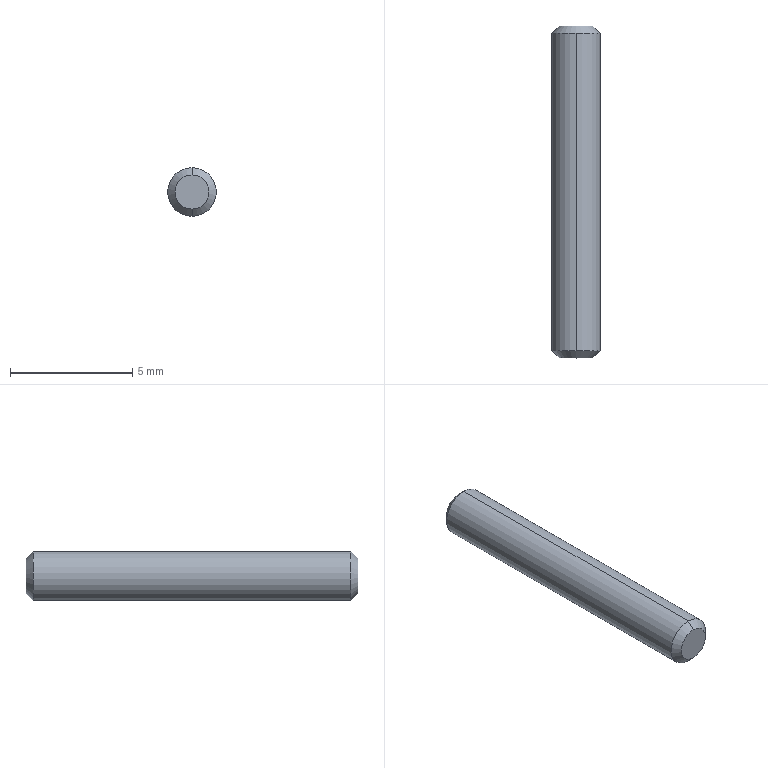Part | SolidWorks | features BaseBody 1 | 1 solid | 8 faces | box 1.99 x 13.6 x 1.99 mm | volume 41.809 mm3 | cone 4 | cylinder 2 | plane 2 | commonest cylinder face diameters 1.99 x2
STEP:
#1=CARTESIAN_POINT('',(0.,19.195,13.599));
#2=VERTEX_POINT('',#1);
#3=CARTESIAN_POINT('',(0.,19.195,11.609));
#4=VERTEX_POINT('',#3);
#5=CARTESIAN_POINT('',(0.,19.195,12.604));
#6=DIRECTION('',(0.,1.,0.));
#7=DIRECTION('',(0.,0.,1.));
#8=AXIS2_PLACEMENT_3D('',#5,#6,#7);
#9=CIRCLE('',#8,0.995);
#10=EDGE_CURVE('',#2,#4,#9,.T.);
#11=ORIENTED_EDGE('',*,*,#10,.T.);
#12=CARTESIAN_POINT('',(0.,32.205,11.609));
#13=VERTEX_POINT('',#12);
#14=CARTESIAN_POINT('',(0.,18.9,11.609));
#15=DIRECTION('',(0.,1.,0.));
#16=VECTOR('',#15,1000.);
#17=LINE('',#14,#16);
#18=EDGE_CURVE('',#4,#13,#17,.T.);
#19=ORIENTED_EDGE('',*,*,#18,.T.);
#20=CARTESIAN_POINT('',(0.,32.205,13.599));
#21=VERTEX_POINT('',#20);
#22=CARTESIAN_POINT('',(0.,32.205,12.604));
#23=DIRECTION('',(0.,-1.,0.));
#24=DIRECTION('',(0.,0.,1.));
#25=AXIS2_PLACEMENT_3D('',#22,#23,#24);
#26=CIRCLE('',#25,0.995);
#27=EDGE_CURVE('',#13,#21,#26,.T.);
#28=ORIENTED_EDGE('',*,*,#27,.T.);
#29=CARTESIAN_POINT('',(0.,18.9,13.599));
#30=DIRECTION('',(0.,1.,0.));
#31=VECTOR('',#30,1000.);
#32=LINE('',#29,#31);
#33=EDGE_CURVE('',#2,#21,#32,.T.);
#34=ORIENTED_EDGE('',*,*,#33,.F.);
#35=EDGE_LOOP('',(#11,#19,#28,#34));
#36=FACE_OUTER_BOUND('',#35,.T.);
#37=CARTESIAN_POINT('',(0.,18.9,12.604));
#38=DIRECTION('',(0.,1.,0.));
#39=DIRECTION('',(0.,0.,1.));
#40=AXIS2_PLACEMENT_3D('',#37,#38,#39);
#41=CYLINDRICAL_SURFACE('',#40,0.995);
#42=ADVANCED_FACE('',(#36),#41,.T.);
#43=CARTESIAN_POINT('',(0.,18.9,13.304));
#44=VERTEX_POINT('',#43);
#45=CARTESIAN_POINT('',(0.,18.9,11.904));
#46=VERTEX_POINT('',#45);
#47=CARTESIAN_POINT('',(0.,18.9,12.604));
#48=DIRECTION('',(0.,1.,0.));
#49=DIRECTION('',(0.,0.,1.));
#50=AXIS2_PLACEMENT_3D('',#47,#48,#49);
#51=CIRCLE('',#50,0.7);
#52=EDGE_CURVE('',#44,#46,#51,.T.);
#53=ORIENTED_EDGE('',*,*,#52,.T.);
#54=CARTESIAN_POINT('',(0.,19.195,11.609));
#55=DIRECTION('',(0.,0.7071,-0.7071));
#56=VECTOR('',#55,1000.);
#57=LINE('',#54,#56);
#58=EDGE_CURVE('',#46,#4,#57,.T.);
#59=ORIENTED_EDGE('',*,*,#58,.T.);
#60=ORIENTED_EDGE('',*,*,#10,.F.);
#61=CARTESIAN_POINT('',(0.,19.195,13.599));
#62=DIRECTION('',(0.,0.7071,0.7071));
#63=VECTOR('',#62,1000.);
#64=LINE('',#61,#63);
#65=EDGE_CURVE('',#44,#2,#64,.T.);
#66=ORIENTED_EDGE('',*,*,#65,.F.);
#67=EDGE_LOOP('',(#53,#59,#60,#66));
#68=FACE_OUTER_BOUND('',#67,.T.);
#69=CARTESIAN_POINT('',(0.,19.195,12.604));
#70=DIRECTION('',(0.,1.,0.));
#71=DIRECTION('',(0.,0.,1.));
#72=AXIS2_PLACEMENT_3D('',#69,#70,#71);
#73=CONICAL_SURFACE('',#72,0.995,0.7854);
#74=ADVANCED_FACE('',(#68),#73,.T.);
#75=CARTESIAN_POINT('',(0.,32.5,11.904));
#76=VERTEX_POINT('',#75);
#77=CARTESIAN_POINT('',(0.,32.5,13.304));
#78=VERTEX_POINT('',#77);
#79=CARTESIAN_POINT('',(0.,32.5,12.604));
#80=DIRECTION('',(0.,-1.,0.));
#81=DIRECTION('',(0.,0.,-1.));
#82=AXIS2_PLACEMENT_3D('',#79,#80,#81);
#83=CIRCLE('',#82,0.7);
#84=EDGE_CURVE('',#76,#78,#83,.T.);
#85=ORIENTED_EDGE('',*,*,#84,.T.);
#86=CARTESIAN_POINT('',(0.,32.205,13.599));
#87=DIRECTION('',(0.,-0.7071,0.7071));
#88=VECTOR('',#87,1000.);
#89=LINE('',#86,#88);
#90=EDGE_CURVE('',#78,#21,#89,.T.);
#91=ORIENTED_EDGE('',*,*,#90,.T.);
#92=ORIENTED_EDGE('',*,*,#27,.F.);
#93=CARTESIAN_POINT('',(0.,32.205,11.609));
#94=DIRECTION('',(0.,-0.7071,-0.7071));
#95=VECTOR('',#94,1000.);
#96=LINE('',#93,#95);
#97=EDGE_CURVE('',#76,#13,#96,.T.);
#98=ORIENTED_EDGE('',*,*,#97,.F.);
#99=EDGE_LOOP('',(#85,#91,#92,#98));
#100=FACE_OUTER_BOUND('',#99,.T.);
#101=CARTESIAN_POINT('',(0.,32.205,12.604));
#102=DIRECTION('',(0.,-1.,0.));
#103=DIRECTION('',(0.,0.,-1.));
#104=AXIS2_PLACEMENT_3D('',#101,#102,#103);
#105=CONICAL_SURFACE('',#104,0.995,0.7854);
#106=ADVANCED_FACE('',(#100),#105,.T.);
#107=ORIENTED_EDGE('',*,*,#18,.F.);
#108=CARTESIAN_POINT('',(0.,19.195,12.604));
#109=DIRECTION('',(0.,1.,0.));
#110=DIRECTION('',(0.,0.,1.));
#111=AXIS2_PLACEMENT_3D('',#108,#109,#110);
#112=CIRCLE('',#111,0.995);
#113=EDGE_CURVE('',#4,#2,#112,.T.);
#114=ORIENTED_EDGE('',*,*,#113,.T.);
#115=ORIENTED_EDGE('',*,*,#33,.T.);
#116=CARTESIAN_POINT('',(0.,32.205,12.604));
#117=DIRECTION('',(0.,-1.,0.));
#118=DIRECTION('',(0.,0.,1.));
#119=AXIS2_PLACEMENT_3D('',#116,#117,#118);
#120=CIRCLE('',#119,0.995);
#121=EDGE_CURVE('',#21,#13,#120,.T.);
#122=ORIENTED_EDGE('',*,*,#121,.T.);
#123=EDGE_LOOP('',(#107,#114,#115,#122));
#124=FACE_OUTER_BOUND('',#123,.T.);
#125=CARTESIAN_POINT('',(0.,18.9,12.604));
#126=DIRECTION('',(0.,1.,0.));
#127=DIRECTION('',(0.,0.,1.));
#128=AXIS2_PLACEMENT_3D('',#125,#126,#127);
#129=CYLINDRICAL_SURFACE('',#128,0.995);
#130=ADVANCED_FACE('',(#124),#129,.T.);
#131=ORIENTED_EDGE('',*,*,#58,.F.);
#132=CARTESIAN_POINT('',(0.,18.9,12.604));
#133=DIRECTION('',(0.,1.,0.));
#134=DIRECTION('',(0.,0.,1.));
#135=AXIS2_PLACEMENT_3D('',#132,#133,#134);
#136=CIRCLE('',#135,0.7);
#137=EDGE_CURVE('',#46,#44,#136,.T.);
#138=ORIENTED_EDGE('',*,*,#137,.T.);
#139=ORIENTED_EDGE('',*,*,#65,.T.);
#140=ORIENTED_EDGE('',*,*,#113,.F.);
#141=EDGE_LOOP('',(#131,#138,#139,#140));
#142=FACE_OUTER_BOUND('',#141,.T.);
#143=CARTESIAN_POINT('',(0.,19.195,12.604));
#144=DIRECTION('',(0.,1.,0.));
#145=DIRECTION('',(0.,0.,1.));
#146=AXIS2_PLACEMENT_3D('',#143,#144,#145);
#147=CONICAL_SURFACE('',#146,0.995,0.7854);
#148=ADVANCED_FACE('',(#142),#147,.T.);
#149=ORIENTED_EDGE('',*,*,#90,.F.);
#150=CARTESIAN_POINT('',(0.,32.5,12.604));
#151=DIRECTION('',(0.,-1.,0.));
#152=DIRECTION('',(0.,0.,-1.));
#153=AXIS2_PLACEMENT_3D('',#150,#151,#152);
#154=CIRCLE('',#153,0.7);
#155=EDGE_CURVE('',#78,#76,#154,.T.);
#156=ORIENTED_EDGE('',*,*,#155,.T.);
#157=ORIENTED_EDGE('',*,*,#97,.T.);
#158=ORIENTED_EDGE('',*,*,#121,.F.);
#159=EDGE_LOOP('',(#149,#156,#157,#158));
#160=FACE_OUTER_BOUND('',#159,.T.);
#161=CARTESIAN_POINT('',(0.,32.205,12.604));
#162=DIRECTION('',(0.,-1.,0.));
#163=DIRECTION('',(0.,0.,-1.));
#164=AXIS2_PLACEMENT_3D('',#161,#162,#163);
#165=CONICAL_SURFACE('',#164,0.995,0.7854);
#166=ADVANCED_FACE('',(#160),#165,.T.);
#167=ORIENTED_EDGE('',*,*,#52,.F.);
#168=ORIENTED_EDGE('',*,*,#137,.F.);
#169=EDGE_LOOP('',(#167,#168));
#170=FACE_OUTER_BOUND('',#169,.T.);
#171=CARTESIAN_POINT('',(0.,18.9,12.604));
#172=DIRECTION('',(0.,1.,0.));
#173=DIRECTION('',(0.,0.,1.));
#174=AXIS2_PLACEMENT_3D('',#171,#172,#173);
#175=PLANE('',#174);
#176=ADVANCED_FACE('',(#170),#175,.F.);
#177=ORIENTED_EDGE('',*,*,#84,.F.);
#178=ORIENTED_EDGE('',*,*,#155,.F.);
#179=EDGE_LOOP('',(#177,#178));
#180=FACE_OUTER_BOUND('',#179,.T.);
#181=CARTESIAN_POINT('',(0.,32.5,12.604));
#182=DIRECTION('',(0.,1.,0.));
#183=DIRECTION('',(0.,0.,1.));
#184=AXIS2_PLACEMENT_3D('',#181,#182,#183);
#185=PLANE('',#184);
#186=ADVANCED_FACE('',(#180),#185,.T.);
#187=CLOSED_SHELL('',(#42,#74,#106,#130,#148,#166,#176,#186));
#188=MANIFOLD_SOLID_BREP('',#187);
#189=CARTESIAN_POINT('',(0.,0.,0.));
#190=DIRECTION('',(0.,0.,1.));
#191=DIRECTION('',(1.,0.,0.));
#192=AXIS2_PLACEMENT_3D('',#189,#190,#191);
#193=(LENGTH_UNIT()NAMED_UNIT(*)SI_UNIT(.MILLI.,.METRE.));
#194=UNCERTAINTY_MEASURE_WITH_UNIT(LENGTH_MEASURE(0.00001),#193,'','');
#195=(NAMED_UNIT(*)PLANE_ANGLE_UNIT()SI_UNIT($,.RADIAN.));
#196=(NAMED_UNIT(*)SI_UNIT($,.STERADIAN.)SOLID_ANGLE_UNIT());
#197=(GEOMETRIC_REPRESENTATION_CONTEXT(3)GLOBAL_UNCERTAINTY_ASSIGNED_CONTEXT((#194))GLOBAL_UNIT_ASSIGNED_CONTEXT((#193,#195,#196))REPRESENTATION_CONTEXT('',''));
#198=ADVANCED_BREP_SHAPE_REPRESENTATION('',(#188,#192),#197);